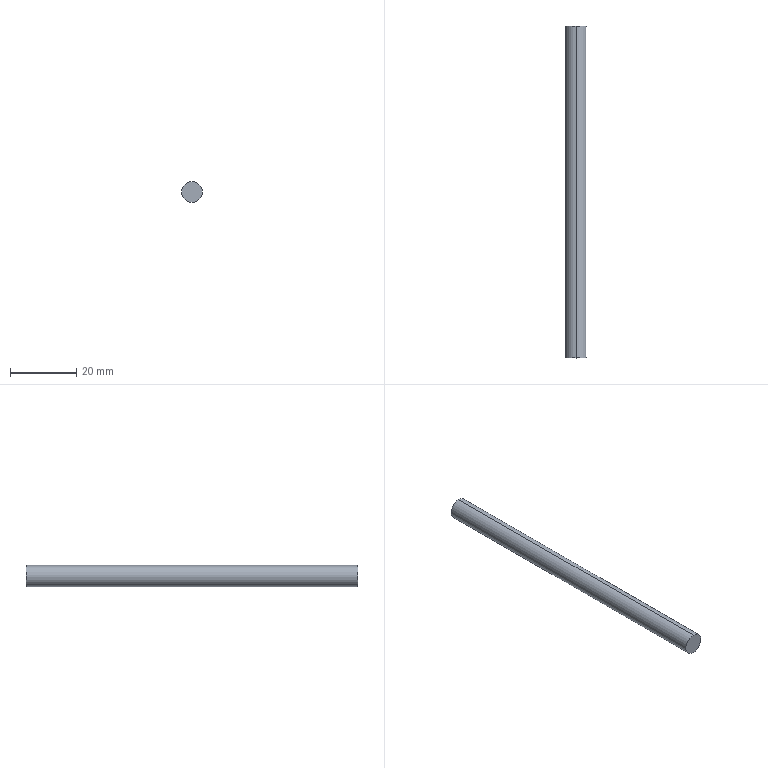Part | SolidWorks | features Extrusion 1 | 1 solid | 4 faces | box 6.35 x 100 x 6.35 mm | volume 3167 mm3 | cylinder 2 | plane 2 | commonest cylinder face diameters 6.35 x2
STEP:
#1=CARTESIAN_POINT('',(0.,100.,3.175));
#2=VERTEX_POINT('',#1);
#3=CARTESIAN_POINT('',(0.,100.,-3.175));
#4=VERTEX_POINT('',#3);
#5=CARTESIAN_POINT('',(0.,100.,0.));
#6=DIRECTION('',(0.,1.,0.));
#7=DIRECTION('',(0.,0.,1.));
#8=AXIS2_PLACEMENT_3D('',#5,#6,#7);
#9=CIRCLE('',#8,3.175);
#10=EDGE_CURVE('',#2,#4,#9,.T.);
#11=ORIENTED_EDGE('',*,*,#10,.F.);
#12=CARTESIAN_POINT('',(0.,0.,3.175));
#13=VERTEX_POINT('',#12);
#14=CARTESIAN_POINT('',(0.,100.,3.175));
#15=DIRECTION('',(0.,-1.,0.));
#16=VECTOR('',#15,1000.);
#17=LINE('',#14,#16);
#18=EDGE_CURVE('',#2,#13,#17,.T.);
#19=ORIENTED_EDGE('',*,*,#18,.T.);
#20=CARTESIAN_POINT('',(0.,0.,-3.175));
#21=VERTEX_POINT('',#20);
#22=CARTESIAN_POINT('',(0.,0.,0.));
#23=DIRECTION('',(0.,1.,0.));
#24=DIRECTION('',(0.,0.,1.));
#25=AXIS2_PLACEMENT_3D('',#22,#23,#24);
#26=CIRCLE('',#25,3.175);
#27=EDGE_CURVE('',#13,#21,#26,.T.);
#28=ORIENTED_EDGE('',*,*,#27,.T.);
#29=CARTESIAN_POINT('',(0.,100.,-3.175));
#30=DIRECTION('',(0.,-1.,0.));
#31=VECTOR('',#30,1000.);
#32=LINE('',#29,#31);
#33=EDGE_CURVE('',#4,#21,#32,.T.);
#34=ORIENTED_EDGE('',*,*,#33,.F.);
#35=EDGE_LOOP('',(#11,#19,#28,#34));
#36=FACE_OUTER_BOUND('',#35,.T.);
#37=CARTESIAN_POINT('',(0.,100.,0.));
#38=DIRECTION('',(0.,-1.,0.));
#39=DIRECTION('',(0.,0.,-1.));
#40=AXIS2_PLACEMENT_3D('',#37,#38,#39);
#41=CYLINDRICAL_SURFACE('',#40,3.175);
#42=ADVANCED_FACE('',(#36),#41,.T.);
#43=ORIENTED_EDGE('',*,*,#18,.F.);
#44=CARTESIAN_POINT('',(0.,100.,0.));
#45=DIRECTION('',(0.,1.,0.));
#46=DIRECTION('',(0.,0.,1.));
#47=AXIS2_PLACEMENT_3D('',#44,#45,#46);
#48=CIRCLE('',#47,3.175);
#49=EDGE_CURVE('',#4,#2,#48,.T.);
#50=ORIENTED_EDGE('',*,*,#49,.F.);
#51=ORIENTED_EDGE('',*,*,#33,.T.);
#52=CARTESIAN_POINT('',(0.,0.,0.));
#53=DIRECTION('',(0.,1.,0.));
#54=DIRECTION('',(0.,0.,1.));
#55=AXIS2_PLACEMENT_3D('',#52,#53,#54);
#56=CIRCLE('',#55,3.175);
#57=EDGE_CURVE('',#21,#13,#56,.T.);
#58=ORIENTED_EDGE('',*,*,#57,.T.);
#59=EDGE_LOOP('',(#43,#50,#51,#58));
#60=FACE_OUTER_BOUND('',#59,.T.);
#61=CARTESIAN_POINT('',(0.,100.,0.));
#62=DIRECTION('',(0.,-1.,0.));
#63=DIRECTION('',(0.,0.,-1.));
#64=AXIS2_PLACEMENT_3D('',#61,#62,#63);
#65=CYLINDRICAL_SURFACE('',#64,3.175);
#66=ADVANCED_FACE('',(#60),#65,.T.);
#67=ORIENTED_EDGE('',*,*,#49,.T.);
#68=ORIENTED_EDGE('',*,*,#10,.T.);
#69=EDGE_LOOP('',(#67,#68));
#70=FACE_OUTER_BOUND('',#69,.T.);
#71=CARTESIAN_POINT('',(0.,100.,0.));
#72=DIRECTION('',(0.,1.,0.));
#73=DIRECTION('',(0.,0.,1.));
#74=AXIS2_PLACEMENT_3D('',#71,#72,#73);
#75=PLANE('',#74);
#76=ADVANCED_FACE('',(#70),#75,.T.);
#77=ORIENTED_EDGE('',*,*,#57,.F.);
#78=ORIENTED_EDGE('',*,*,#27,.F.);
#79=EDGE_LOOP('',(#77,#78));
#80=FACE_OUTER_BOUND('',#79,.T.);
#81=CARTESIAN_POINT('',(0.,0.,0.));
#82=DIRECTION('',(0.,1.,0.));
#83=DIRECTION('',(0.,0.,1.));
#84=AXIS2_PLACEMENT_3D('',#81,#82,#83);
#85=PLANE('',#84);
#86=ADVANCED_FACE('',(#80),#85,.F.);
#87=CLOSED_SHELL('',(#42,#66,#76,#86));
#88=MANIFOLD_SOLID_BREP('',#87);
#89=CARTESIAN_POINT('',(0.,0.,0.));
#90=DIRECTION('',(0.,0.,1.));
#91=DIRECTION('',(1.,0.,0.));
#92=AXIS2_PLACEMENT_3D('',#89,#90,#91);
#93=(LENGTH_UNIT()NAMED_UNIT(*)SI_UNIT(.MILLI.,.METRE.));
#94=UNCERTAINTY_MEASURE_WITH_UNIT(LENGTH_MEASURE(0.00001),#93,'','');
#95=(NAMED_UNIT(*)PLANE_ANGLE_UNIT()SI_UNIT($,.RADIAN.));
#96=(NAMED_UNIT(*)SI_UNIT($,.STERADIAN.)SOLID_ANGLE_UNIT());
#97=(GEOMETRIC_REPRESENTATION_CONTEXT(3)GLOBAL_UNCERTAINTY_ASSIGNED_CONTEXT((#94))GLOBAL_UNIT_ASSIGNED_CONTEXT((#93,#95,#96))REPRESENTATION_CONTEXT('',''));
#98=ADVANCED_BREP_SHAPE_REPRESENTATION('',(#88,#92),#97);